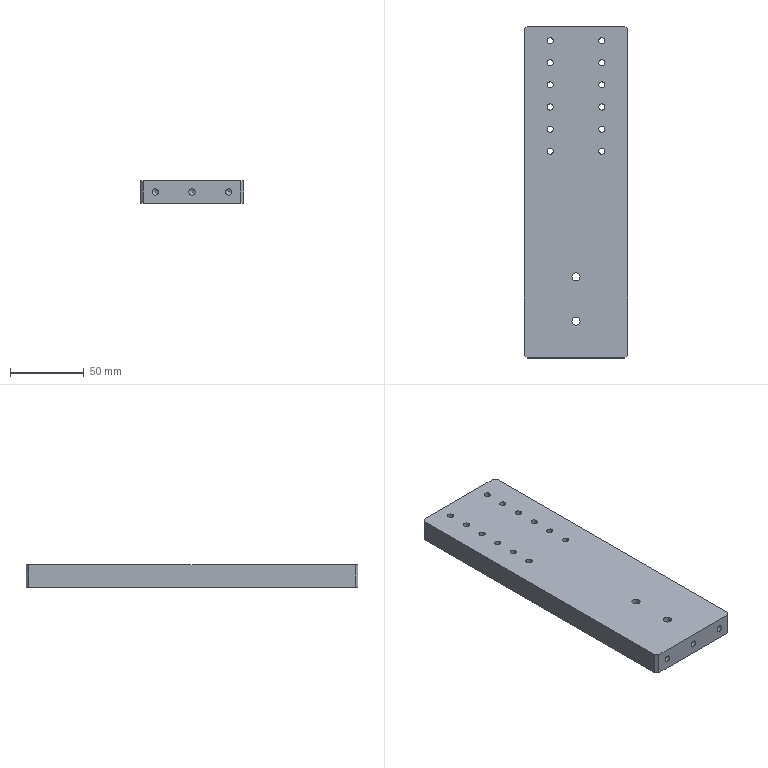CAM job | NX | 3-axis milling, drilling | part box 70 x 225 x 15 mm | stock box 75 x 230 x 20 mm
Tools:
number,name,description,diameter,corner_radius,flute_length,length,flutes
6,D6,平底铣刀-粗,6.0,0.0,25.0,75.0,2
9,D10,平底铣刀-粗,10.0,0.0,35.0,75.0,2
18,D4-J,平底铣刀-精,4.0,0.0,50.0,75.0,2
7,D6-J,平底铣刀-精,6.0,0.0,25.0,75.0,2
10,D10-J,平底铣刀-精,10.0,0.0,35.0,75.0,2
1,D80R0.8飞刀,圆鼻刀-粗,80.0,0.8,50.0,75.0,2
1,D80R0.8飞刀-J,圆鼻刀-精,80.0,0.8,50.0,75.0,2
2,D6倒角刀,倒角刀,6.0,0.0,3.0,25.0,2
22,M5X0.8,丝锥,4.2,0.0,35.0,50.0,2
17,ZT5.5,钻头,5.5,0.0,35.0,50.0,2
14,钻头4.2,Twist Drill 4.2 mm,4.2,0.0,41.0,41.738,2
Operations:
program,operation,operation_type,tool,method,geometry_group,spindle_rpm,surface_speed,feed_per_tooth,feed_cut,feed_plunge,cut_length_mm,path_length_mm,cut_time_min,machine_time_min
B,底壁铣飞面一刀开粗_COPY,VolumeBased25DMillingOperation,D80R0.8飞刀,分层开粗-切深K-步距G,W-B,5000.0,1256.637,0.3,3000.0,100.0,3331.94,6524.137,1.111,1.43
B,底壁铣飞面一刀精光_COPY,VolumeBased25DMillingOperation,D80R0.8飞刀-J,侧刃精光-切深K-步距G,W-B,5000.0,1256.637,0.1,1000.0,100.0,332.998,368.998,0.333,0.3366
B,钻倒角_1,Operation,D6倒角刀,METHOD,W-B,8000.0,150.796,0.0625,1000.0,0.0,68.4,397.899,0.0684,0.1013
B,平面去毛刺6X45L_COPY,SurfaceContour,D6倒角刀,爬面_倒角-切深0-步距G,W-B,6500.0,122.519,0.1154,1500.0,100.0,624.915,828.719,0.4166,0.437
A,顶面,FaceMilling,D80R0.8飞刀,侧刃精光-切深K-步距G,W-A,4000.0,1005.28,0.125,1000.0,100.0,319.0,355.0,0.319,0.3226
A,外形粗_2,VolumeBased25DMillingOperation,D10,METHOD,W-A,8000.0,251.327,0.3125,5000.0,80.0,20374.319,20428.019,4.075,4.08
A,台阶粗_2,CavityMilling,D10,METHOD,W-A,6000.0,188.0,0.25,3500.0,100.0,7050.821,7247.435,2.014,2.034
A,打点-深0.8,Operation,D6倒角刀,NONE,W-A,8000.0,150.796,0.0312,500.0,90.0,25.2,408.639,0.0504,0.0887
A,通孔-M5螺纹底孔,Operation,钻头4.2,NONE,W-A,3000.0,39.584,0.0583,350.0,90.0,243.142,728.631,0.6947,0.7432
A,沉头孔-钻孔0段,Operation,ZT5.5,NONE,W-A,1200.0,20.735,0.0625,150.0,90.0,39.305,149.626,0.262,0.2731
A,铣孔开粗D6_1,CylinderMilling,D6,NONE,W-A,8000.0,150.796,0.075,1200.0,100.0,394.27,517.27,0.3286,0.3409
A,铣孔精光D6_1,CylinderMilling,D6-J,精光步距切深关,W-A,8000.0,150.792,0.0625,1000.0,100.0,75.453,199.453,0.1509,0.1633
A,底精_1,VolumeBased25DMillingOperation,D6-J,METHOD,W-A,6000.0,113.0,0.2083,1200.0,100.0,1719.9,1764.9,1.433,1.438
A,清角D4,ZLevelMilling,D4-J,METHOD,W-A,6000.0,75.0,0.25,2500.0,80.0,218.499,317.582,0.0876,0.0975
A,仅选体,SurfaceContour,D6倒角刀,METHOD,W-A,8000.0,150.796,0.1875,3000.0,100.0,908.792,1112.632,0.3029,0.3233
A,铣倒角_1,PlanarMilling,D6倒角刀,METHOD,W-A,8000.0,150.796,0.0312,500.0,100.0,216.244,965.272,0.4325,0.5074
A,铣倒角_2,PlanarMilling,D6倒角刀,NONE,W-A,8000.0,150.796,0.05,800.0,100.0,80.502,179.52,0.1006,0.1105
A,通孔-攻牙M5,Operation,M5X0.8,METHOD,W-A,500.0,6.597,0.0008,0.8,90.0,198.0,638.347,247.5,247.544
A,底侧精_3,VolumeBased25DMillingOperation,D6-J,METHOD,W-A,6000.0,113.0,0.2083,1200.0,100.0,297.742,342.732,0.2481,0.2526
A,外形半精_2,VolumeBased25DMillingOperation,D10-J,METHOD,W-A,8000.0,251.327,0.0625,1000.0,100.0,621.688,691.088,0.6217,0.6286